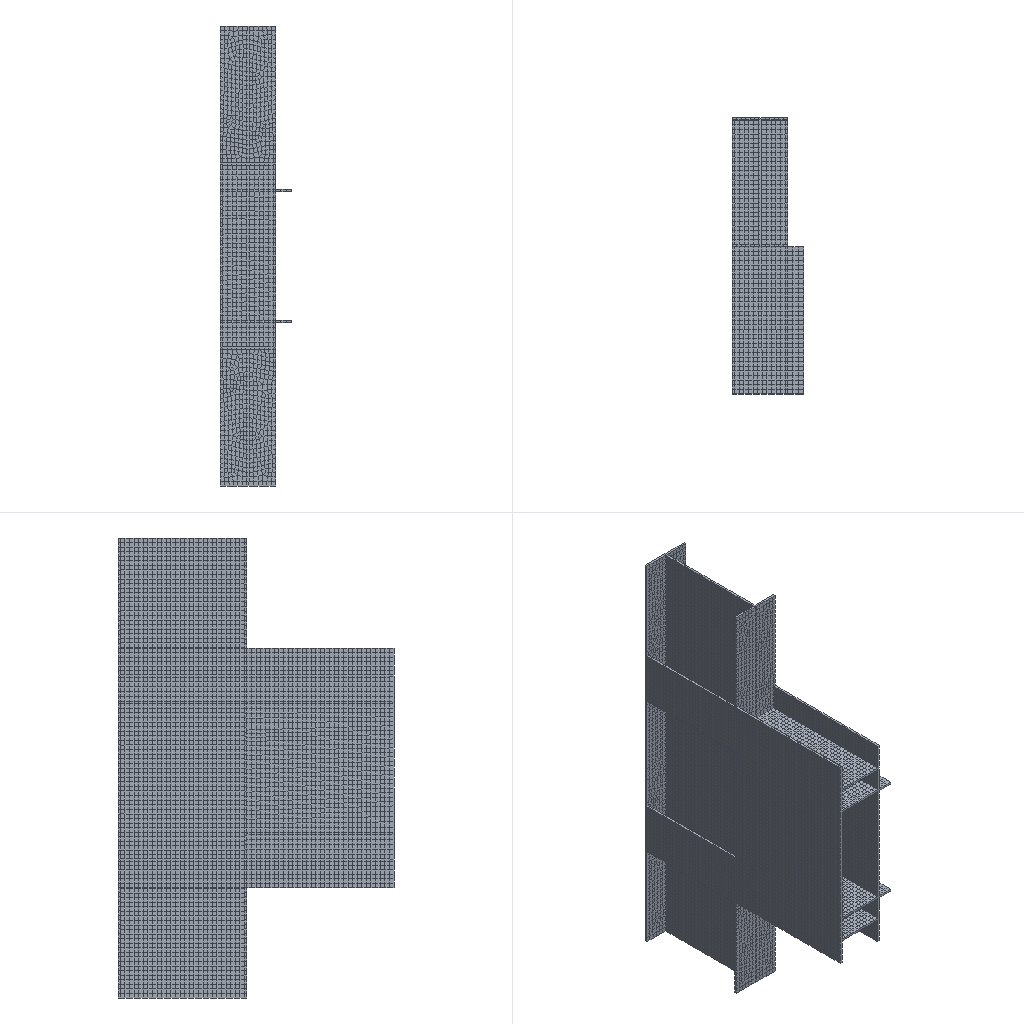Simulation study | abaqus
Set-up summary:
category,name,step,type,value,unit,region
solver,abaqus
solver,version,,,Abaqus/Standard 2020
units,not stated in the deck,,not stated
analysis,deck,,static,static
load_step,Step-1,Step-1,static,nlgeom=True
contact,interactions,,,general=0 pairs=0 ties=0
load_step,requested,,,1
mesh,nodes,,,25546
mesh,elements,,,12747
element_type,C3D8R,,solid,12747
load,load commands in deck,,count,1
bc,support commands in deck,,count,1
material,MATERIAL-1,,in results
check,setup vs results,,match,"per instance, exact: element labels, types and connectivity; labels of the nodes the elements use; coordinates of those nodes at SINGLE_PRECISION in 1 of 1 instance(s)"
Abaqus input file, long lists of numbers shortened:
*Heading
** Job name: Job-2 Model name: Model-1-Copy
** Generated by: Abaqus/CAE 2020
*Preprint, echo=NO, model=NO, history=NO, contact=NO
**
** PARTS
**
*Part, name=Part-3
*Node
      1,           5.,        -540.,        1280.
      2,          -5.,        -540.,        1280.
** (25544 more lines like these left out)
*Element, type=C3D8R
 1,   4,   3,   2,   1, 265, 266, 275, 276
 2,   6, 252, 245,   5,   9, 261, 280,  12
** (12745 more lines like these left out)
*Nset, nset=Set-2, generate
     1,  25546,      1
*Elset, elset=Set-2, generate
     1,  12747,      1
** Section: Section-1
*Solid Section, elset=Set-2, material=Material-1
,
*End Part
**
**
** ASSEMBLY
**
*Assembly, name=Assembly
**
*Instance, name=Part-3-1, part=Part-3
*End Instance
**
*Nset, nset=Set-1, instance=Part-3-1
   13,   14,   15,   16,   45,   46,   47,   48,   84,   85,   86,   87,   88,   89,   90,   91
  139,  140,  141,  142,  143,  144,  209,  210,  211,  212,  213,  214,  215,  216,  217,  218
** (18 more lines like these left out)
*Elset, elset=Set-1, instance=Part-3-1
   353,   354,   355,   356,   357,   358,   359,   360,   361,   362,   363,   596,   597,   598,   599,   600
   601,   931,   932,   933,   934,   935,   936,   937,  3740,  3741,  3742,  3743,  3744,  3745,  3746,  8870
** (8 more lines like these left out)
*Nset, nset=Set-2, instance=Part-3-1, generate
     1,  25546,      1
*Elset, elset=Set-2, instance=Part-3-1, generate
     1,  12747,      1
*End Assembly
*Amplitude, name=Amp-1
             0.,              0.,             0.5,              1.
**
** MATERIALS
**
*Material, name=Material-1
*Density
 7.8e-09,
*Elastic
210000., 0.3
*Expansion
 1e-05,
*Plastic
365.,    0.
398., 0.005
432., 0.011
**
** PREDEFINED FIELDS
**
** Name: Predefined Field-1   Type: Temperature
*Initial Conditions, type=TEMPERATURE
Set-2, 25.
** ----------------------------------------------------------------
**
** STEP: Step-1
**
*Step, name=Step-1, nlgeom=YES, inc=1000
*Static, stabilize=0.0002, allsdtol=0.05, continue=NO
0.01, 1., 1e-05, 0.1
**
** BOUNDARY CONDITIONS
**
** Name: BC-1 Type: 对称/反对称/完全固定
*Boundary
Set-1, ENCASTRE
**
** PREDEFINED FIELDS
**
** Name: Predefined Field-1   Type: Temperature
*Temperature, amplitude=Amp-1
Set-2, -200.
**
** OUTPUT REQUESTS
**
*Restart, write, frequency=0
**
** FIELD OUTPUT: F-Output-1
**
*Output, field
*Node Output
CF, NT, RF, RM, RT, U, V
*Element Output, directions=YES
E, LE, MISES, MISESMAX, MISESONLY, PE, PEEQ, PEEQMAX, PEEQT, PEMAG, PEQC, PRESSONLY, S, SEQUT, SSAVG, TEMP
*Contact Output
CDISP, CSTRESS
**
** HISTORY OUTPUT: H-Output-1
**
*Output, history, variable=PRESELECT
*End Step
Results summary:
result,step,,completed,increments=15 time=1.0/1.0
result,analysis,,,static
result,last_loadstep,,,1
result,analysis steps,,count,1
result,primary field,,,U
result,reaction total,,FX,0.000458,model units
result,reaction total,,FY,0.01093,model units
result,reaction total,,FZ,-0.002315,model units